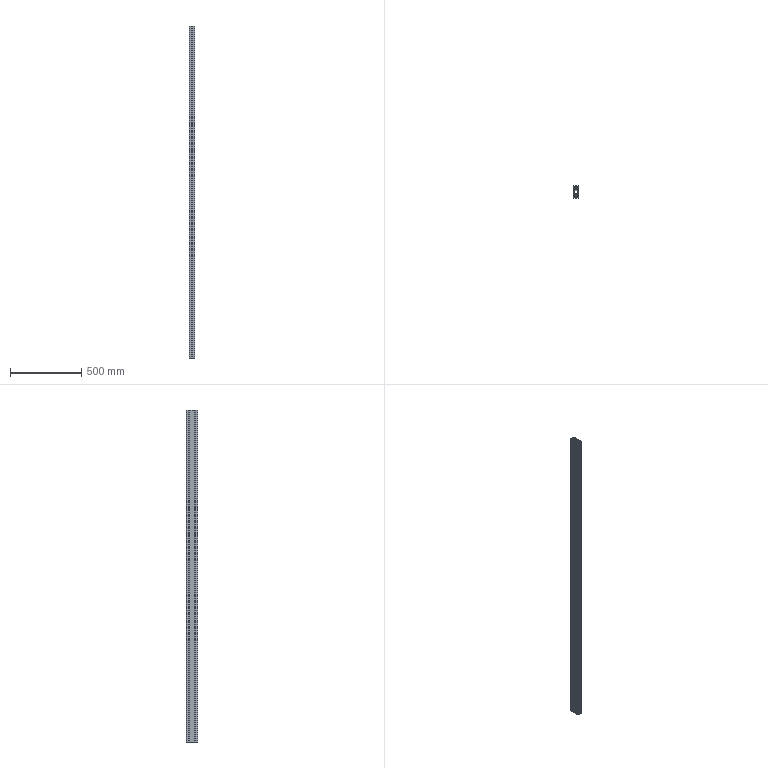Part | NX | features BREP 1 | 1 solid | 182 faces | box 40 x 80 x 2324 mm | volume 2589521 mm3 | plane 112 | cylinder 70 | commonest cylinder face diameters 2 x36 0.76 x20 10.5 x10 6 x4